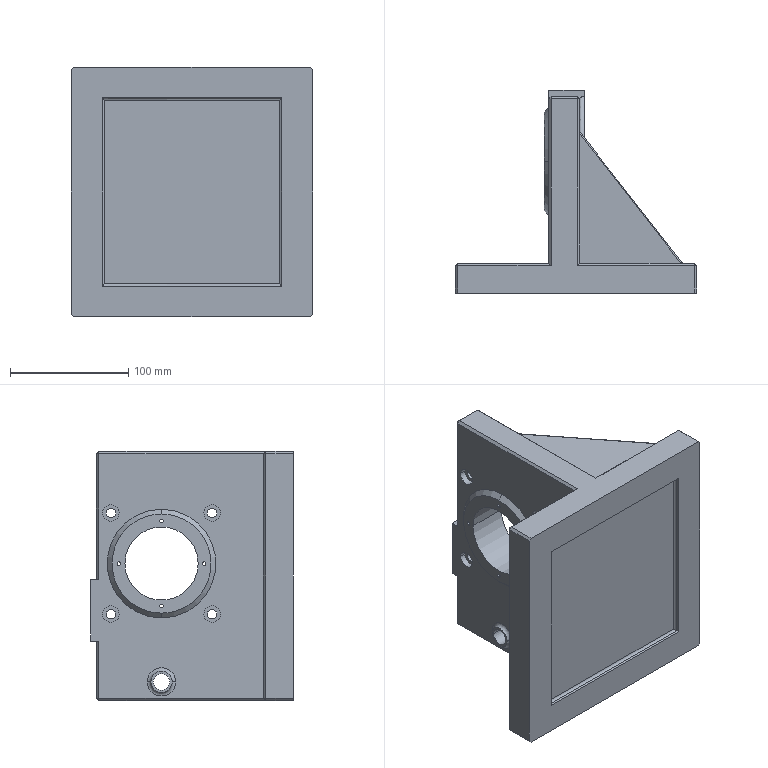Part | SolidWorks | features ICE 19, Fillet 5, Chamfer 3, Extrusion 1 | 1 solid | 126 faces | box 204 x 171.5 x 211 mm | volume 1841584 mm3 | plane 65 | cylinder 46 | torus 12 | cone 2 | spline 1 | commonest cylinder face diameters 14 x10 2 x8 3 x8 8 x8 2.5 x4 4 x4